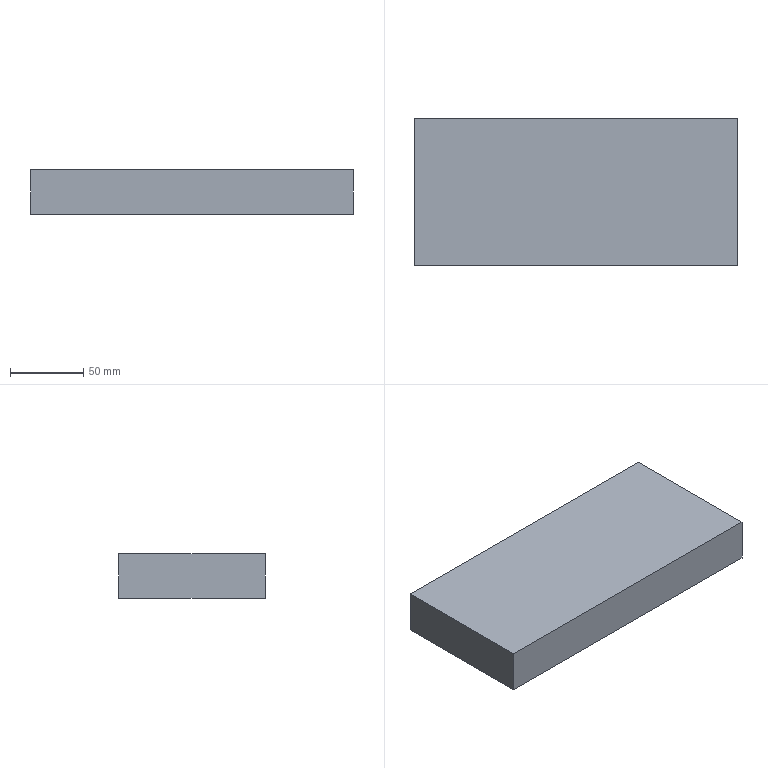Part | SolidWorks | features Extrusion 1 | 1 solid | 6 faces | box 220 x 100 x 30 mm | volume 660000 mm3 | plane 6
STEP:
#1=CARTESIAN_POINT('',(110.,0.,15.));
#2=VERTEX_POINT('',#1);
#3=CARTESIAN_POINT('',(110.,0.,-15.));
#4=VERTEX_POINT('',#3);
#5=CARTESIAN_POINT('',(110.,0.,15.));
#6=DIRECTION('',(0.,0.,-1.));
#7=VECTOR('',#6,1000.);
#8=LINE('',#5,#7);
#9=EDGE_CURVE('',#2,#4,#8,.T.);
#10=ORIENTED_EDGE('',*,*,#9,.T.);
#11=CARTESIAN_POINT('',(110.,100.,-15.));
#12=VERTEX_POINT('',#11);
#13=CARTESIAN_POINT('',(110.,100.,-15.));
#14=DIRECTION('',(0.,-1.,0.));
#15=VECTOR('',#14,1000.);
#16=LINE('',#13,#15);
#17=EDGE_CURVE('',#12,#4,#16,.T.);
#18=ORIENTED_EDGE('',*,*,#17,.F.);
#19=CARTESIAN_POINT('',(110.,100.,15.));
#20=VERTEX_POINT('',#19);
#21=CARTESIAN_POINT('',(110.,100.,15.));
#22=DIRECTION('',(0.,0.,-1.));
#23=VECTOR('',#22,1000.);
#24=LINE('',#21,#23);
#25=EDGE_CURVE('',#20,#12,#24,.T.);
#26=ORIENTED_EDGE('',*,*,#25,.F.);
#27=CARTESIAN_POINT('',(110.,100.,15.));
#28=DIRECTION('',(0.,-1.,0.));
#29=VECTOR('',#28,1000.);
#30=LINE('',#27,#29);
#31=EDGE_CURVE('',#20,#2,#30,.T.);
#32=ORIENTED_EDGE('',*,*,#31,.T.);
#33=EDGE_LOOP('',(#10,#18,#26,#32));
#34=FACE_OUTER_BOUND('',#33,.T.);
#35=CARTESIAN_POINT('',(110.,100.,15.));
#36=DIRECTION('',(-1.,0.,0.));
#37=DIRECTION('',(0.,0.,1.));
#38=AXIS2_PLACEMENT_3D('',#35,#36,#37);
#39=PLANE('',#38);
#40=ADVANCED_FACE('',(#34),#39,.F.);
#41=CARTESIAN_POINT('',(-110.,0.,-15.));
#42=VERTEX_POINT('',#41);
#43=CARTESIAN_POINT('',(-110.,0.,-15.));
#44=DIRECTION('',(-1.,0.,0.));
#45=VECTOR('',#44,1000.);
#46=LINE('',#43,#45);
#47=EDGE_CURVE('',#4,#42,#46,.T.);
#48=ORIENTED_EDGE('',*,*,#47,.T.);
#49=CARTESIAN_POINT('',(-110.,100.,-15.));
#50=VERTEX_POINT('',#49);
#51=CARTESIAN_POINT('',(-110.,100.,-15.));
#52=DIRECTION('',(0.,-1.,0.));
#53=VECTOR('',#52,1000.);
#54=LINE('',#51,#53);
#55=EDGE_CURVE('',#50,#42,#54,.T.);
#56=ORIENTED_EDGE('',*,*,#55,.F.);
#57=CARTESIAN_POINT('',(-110.,100.,-15.));
#58=DIRECTION('',(-1.,0.,0.));
#59=VECTOR('',#58,1000.);
#60=LINE('',#57,#59);
#61=EDGE_CURVE('',#12,#50,#60,.T.);
#62=ORIENTED_EDGE('',*,*,#61,.F.);
#63=ORIENTED_EDGE('',*,*,#17,.T.);
#64=EDGE_LOOP('',(#48,#56,#62,#63));
#65=FACE_OUTER_BOUND('',#64,.T.);
#66=CARTESIAN_POINT('',(-110.,100.,-15.));
#67=DIRECTION('',(0.,0.,1.));
#68=DIRECTION('',(1.,0.,0.));
#69=AXIS2_PLACEMENT_3D('',#66,#67,#68);
#70=PLANE('',#69);
#71=ADVANCED_FACE('',(#65),#70,.F.);
#72=CARTESIAN_POINT('',(-110.,0.,15.));
#73=VERTEX_POINT('',#72);
#74=CARTESIAN_POINT('',(-110.,0.,15.));
#75=DIRECTION('',(0.,0.,1.));
#76=VECTOR('',#75,1000.);
#77=LINE('',#74,#76);
#78=EDGE_CURVE('',#42,#73,#77,.T.);
#79=ORIENTED_EDGE('',*,*,#78,.T.);
#80=CARTESIAN_POINT('',(-110.,100.,15.));
#81=VERTEX_POINT('',#80);
#82=CARTESIAN_POINT('',(-110.,100.,15.));
#83=DIRECTION('',(0.,-1.,0.));
#84=VECTOR('',#83,1000.);
#85=LINE('',#82,#84);
#86=EDGE_CURVE('',#81,#73,#85,.T.);
#87=ORIENTED_EDGE('',*,*,#86,.F.);
#88=CARTESIAN_POINT('',(-110.,100.,15.));
#89=DIRECTION('',(0.,0.,1.));
#90=VECTOR('',#89,1000.);
#91=LINE('',#88,#90);
#92=EDGE_CURVE('',#50,#81,#91,.T.);
#93=ORIENTED_EDGE('',*,*,#92,.F.);
#94=ORIENTED_EDGE('',*,*,#55,.T.);
#95=EDGE_LOOP('',(#79,#87,#93,#94));
#96=FACE_OUTER_BOUND('',#95,.T.);
#97=CARTESIAN_POINT('',(-110.,100.,15.));
#98=DIRECTION('',(1.,0.,0.));
#99=DIRECTION('',(0.,0.,-1.));
#100=AXIS2_PLACEMENT_3D('',#97,#98,#99);
#101=PLANE('',#100);
#102=ADVANCED_FACE('',(#96),#101,.F.);
#103=CARTESIAN_POINT('',(-110.,0.,15.));
#104=DIRECTION('',(1.,0.,0.));
#105=VECTOR('',#104,1000.);
#106=LINE('',#103,#105);
#107=EDGE_CURVE('',#73,#2,#106,.T.);
#108=ORIENTED_EDGE('',*,*,#107,.T.);
#109=ORIENTED_EDGE('',*,*,#31,.F.);
#110=CARTESIAN_POINT('',(-110.,100.,15.));
#111=DIRECTION('',(1.,0.,0.));
#112=VECTOR('',#111,1000.);
#113=LINE('',#110,#112);
#114=EDGE_CURVE('',#81,#20,#113,.T.);
#115=ORIENTED_EDGE('',*,*,#114,.F.);
#116=ORIENTED_EDGE('',*,*,#86,.T.);
#117=EDGE_LOOP('',(#108,#109,#115,#116));
#118=FACE_OUTER_BOUND('',#117,.T.);
#119=CARTESIAN_POINT('',(-110.,100.,15.));
#120=DIRECTION('',(0.,0.,-1.));
#121=DIRECTION('',(-1.,0.,0.));
#122=AXIS2_PLACEMENT_3D('',#119,#120,#121);
#123=PLANE('',#122);
#124=ADVANCED_FACE('',(#118),#123,.F.);
#125=ORIENTED_EDGE('',*,*,#25,.T.);
#126=ORIENTED_EDGE('',*,*,#61,.T.);
#127=ORIENTED_EDGE('',*,*,#92,.T.);
#128=ORIENTED_EDGE('',*,*,#114,.T.);
#129=EDGE_LOOP('',(#125,#126,#127,#128));
#130=FACE_OUTER_BOUND('',#129,.T.);
#131=CARTESIAN_POINT('',(0.,100.,0.));
#132=DIRECTION('',(0.,-1.,0.));
#133=DIRECTION('',(0.,0.,-1.));
#134=AXIS2_PLACEMENT_3D('',#131,#132,#133);
#135=PLANE('',#134);
#136=ADVANCED_FACE('',(#130),#135,.F.);
#137=ORIENTED_EDGE('',*,*,#9,.F.);
#138=ORIENTED_EDGE('',*,*,#107,.F.);
#139=ORIENTED_EDGE('',*,*,#78,.F.);
#140=ORIENTED_EDGE('',*,*,#47,.F.);
#141=EDGE_LOOP('',(#137,#138,#139,#140));
#142=FACE_OUTER_BOUND('',#141,.T.);
#143=CARTESIAN_POINT('',(0.,0.,0.));
#144=DIRECTION('',(0.,-1.,0.));
#145=DIRECTION('',(0.,0.,-1.));
#146=AXIS2_PLACEMENT_3D('',#143,#144,#145);
#147=PLANE('',#146);
#148=ADVANCED_FACE('',(#142),#147,.T.);
#149=CLOSED_SHELL('',(#40,#71,#102,#124,#136,#148));
#150=MANIFOLD_SOLID_BREP('',#149);
#151=CARTESIAN_POINT('',(0.,0.,0.));
#152=DIRECTION('',(0.,0.,1.));
#153=DIRECTION('',(1.,0.,0.));
#154=AXIS2_PLACEMENT_3D('',#151,#152,#153);
#155=(LENGTH_UNIT()NAMED_UNIT(*)SI_UNIT(.MILLI.,.METRE.));
#156=UNCERTAINTY_MEASURE_WITH_UNIT(LENGTH_MEASURE(0.00001),#155,'','');
#157=(NAMED_UNIT(*)PLANE_ANGLE_UNIT()SI_UNIT($,.RADIAN.));
#158=(NAMED_UNIT(*)SI_UNIT($,.STERADIAN.)SOLID_ANGLE_UNIT());
#159=(GEOMETRIC_REPRESENTATION_CONTEXT(3)GLOBAL_UNCERTAINTY_ASSIGNED_CONTEXT((#156))GLOBAL_UNIT_ASSIGNED_CONTEXT((#155,#157,#158))REPRESENTATION_CONTEXT('',''));
#160=ADVANCED_BREP_SHAPE_REPRESENTATION('',(#150,#154),#159);